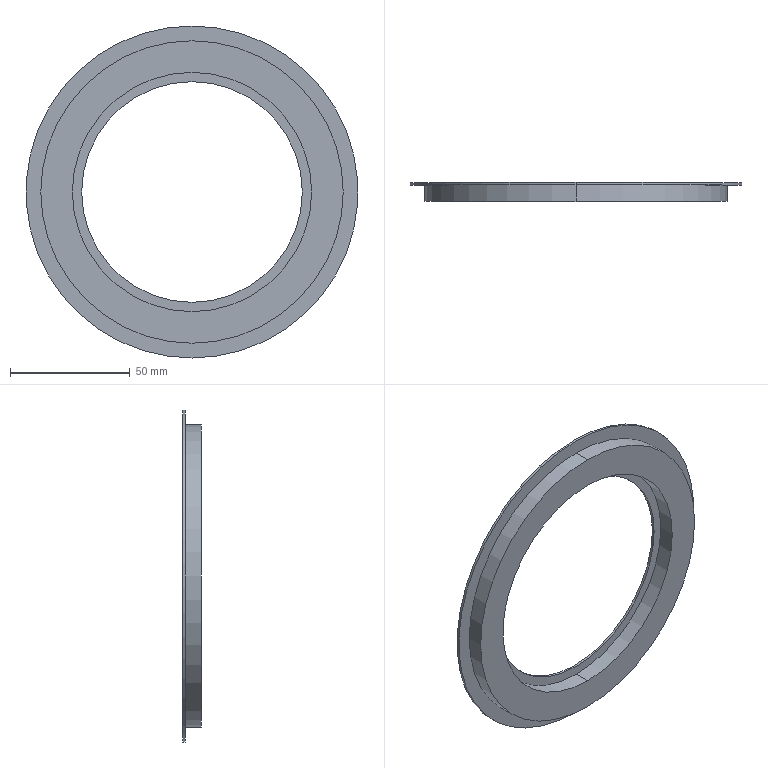Part | SolidWorks | features Revolution 1 | 2 solids | 18 faces | box 138.727 x 7.789 x 138.727 mm | volume 36485 mm3 | cylinder 12 | plane 6 | commonest cylinder face diameters 92.162 x2 100 x2 103.706 x2 124.067 x2 126.387 x2 138.727 x2
STEP:
#1=CARTESIAN_POINT('',(0.,160.532,69.363));
#2=VERTEX_POINT('',#1);
#3=CARTESIAN_POINT('',(0.,160.532,-69.363));
#4=VERTEX_POINT('',#3);
#5=CARTESIAN_POINT('',(0.,160.532,0.));
#6=DIRECTION('',(0.,1.,0.));
#7=DIRECTION('',(0.,0.,1.));
#8=AXIS2_PLACEMENT_3D('',#5,#6,#7);
#9=CIRCLE('',#8,69.363);
#10=EDGE_CURVE('',#2,#4,#9,.T.);
#11=ORIENTED_EDGE('',*,*,#10,.T.);
#12=CARTESIAN_POINT('',(0.,161.532,-69.363));
#13=VERTEX_POINT('',#12);
#14=CARTESIAN_POINT('',(0.,0.,-69.363));
#15=DIRECTION('',(0.,1.,0.));
#16=VECTOR('',#15,1000.);
#17=LINE('',#14,#16);
#18=EDGE_CURVE('',#4,#13,#17,.T.);
#19=ORIENTED_EDGE('',*,*,#18,.T.);
#20=CARTESIAN_POINT('',(0.,161.532,69.363));
#21=VERTEX_POINT('',#20);
#22=CARTESIAN_POINT('',(0.,161.532,0.));
#23=DIRECTION('',(0.,1.,0.));
#24=DIRECTION('',(0.,0.,1.));
#25=AXIS2_PLACEMENT_3D('',#22,#23,#24);
#26=CIRCLE('',#25,69.363);
#27=EDGE_CURVE('',#21,#13,#26,.T.);
#28=ORIENTED_EDGE('',*,*,#27,.F.);
#29=CARTESIAN_POINT('',(0.,0.,69.363));
#30=DIRECTION('',(0.,1.,0.));
#31=VECTOR('',#30,1000.);
#32=LINE('',#29,#31);
#33=EDGE_CURVE('',#2,#21,#32,.T.);
#34=ORIENTED_EDGE('',*,*,#33,.F.);
#35=EDGE_LOOP('',(#11,#19,#28,#34));
#36=FACE_OUTER_BOUND('',#35,.T.);
#37=CARTESIAN_POINT('',(0.,0.,0.));
#38=DIRECTION('',(0.,1.,0.));
#39=DIRECTION('',(0.,0.,1.));
#40=AXIS2_PLACEMENT_3D('',#37,#38,#39);
#41=CYLINDRICAL_SURFACE('',#40,69.363);
#42=ADVANCED_FACE('',(#36),#41,.T.);
#43=CARTESIAN_POINT('',(0.,160.532,-62.034));
#44=VERTEX_POINT('',#43);
#45=CARTESIAN_POINT('',(0.,160.532,62.034));
#46=VERTEX_POINT('',#45);
#47=CARTESIAN_POINT('',(0.,160.532,0.));
#48=DIRECTION('',(0.,1.,0.));
#49=DIRECTION('',(0.,0.,1.));
#50=AXIS2_PLACEMENT_3D('',#47,#48,#49);
#51=CIRCLE('',#50,62.034);
#52=EDGE_CURVE('',#44,#46,#51,.T.);
#53=ORIENTED_EDGE('',*,*,#52,.F.);
#54=CARTESIAN_POINT('',(0.,161.532,-62.034));
#55=VERTEX_POINT('',#54);
#56=CARTESIAN_POINT('',(0.,0.,-62.034));
#57=DIRECTION('',(0.,1.,0.));
#58=VECTOR('',#57,1000.);
#59=LINE('',#56,#58);
#60=EDGE_CURVE('',#44,#55,#59,.T.);
#61=ORIENTED_EDGE('',*,*,#60,.T.);
#62=CARTESIAN_POINT('',(0.,161.532,62.034));
#63=VERTEX_POINT('',#62);
#64=CARTESIAN_POINT('',(0.,161.532,0.));
#65=DIRECTION('',(0.,1.,0.));
#66=DIRECTION('',(0.,0.,1.));
#67=AXIS2_PLACEMENT_3D('',#64,#65,#66);
#68=CIRCLE('',#67,62.034);
#69=EDGE_CURVE('',#55,#63,#68,.T.);
#70=ORIENTED_EDGE('',*,*,#69,.T.);
#71=CARTESIAN_POINT('',(0.,0.,62.034));
#72=DIRECTION('',(0.,1.,0.));
#73=VECTOR('',#72,1000.);
#74=LINE('',#71,#73);
#75=EDGE_CURVE('',#46,#63,#74,.T.);
#76=ORIENTED_EDGE('',*,*,#75,.F.);
#77=EDGE_LOOP('',(#53,#61,#70,#76));
#78=FACE_OUTER_BOUND('',#77,.T.);
#79=CARTESIAN_POINT('',(0.,0.,0.));
#80=DIRECTION('',(0.,1.,0.));
#81=DIRECTION('',(0.,0.,1.));
#82=AXIS2_PLACEMENT_3D('',#79,#80,#81);
#83=CYLINDRICAL_SURFACE('',#82,62.034);
#84=ADVANCED_FACE('',(#78),#83,.F.);
#85=CARTESIAN_POINT('',(0.,153.779,-50.));
#86=VERTEX_POINT('',#85);
#87=CARTESIAN_POINT('',(0.,153.779,50.));
#88=VERTEX_POINT('',#87);
#89=CARTESIAN_POINT('',(0.,153.779,0.));
#90=DIRECTION('',(0.,1.,0.));
#91=DIRECTION('',(0.,0.,1.));
#92=AXIS2_PLACEMENT_3D('',#89,#90,#91);
#93=CIRCLE('',#92,50.);
#94=EDGE_CURVE('',#86,#88,#93,.T.);
#95=ORIENTED_EDGE('',*,*,#94,.F.);
#96=CARTESIAN_POINT('',(0.,160.532,-50.));
#97=VERTEX_POINT('',#96);
#98=CARTESIAN_POINT('',(0.,0.,-50.));
#99=DIRECTION('',(0.,1.,0.));
#100=VECTOR('',#99,1000.);
#101=LINE('',#98,#100);
#102=EDGE_CURVE('',#86,#97,#101,.T.);
#103=ORIENTED_EDGE('',*,*,#102,.T.);
#104=CARTESIAN_POINT('',(0.,160.532,50.));
#105=VERTEX_POINT('',#104);
#106=CARTESIAN_POINT('',(0.,160.532,0.));
#107=DIRECTION('',(0.,1.,0.));
#108=DIRECTION('',(0.,0.,1.));
#109=AXIS2_PLACEMENT_3D('',#106,#107,#108);
#110=CIRCLE('',#109,50.);
#111=EDGE_CURVE('',#97,#105,#110,.T.);
#112=ORIENTED_EDGE('',*,*,#111,.T.);
#113=CARTESIAN_POINT('',(0.,0.,50.));
#114=DIRECTION('',(0.,1.,0.));
#115=VECTOR('',#114,1000.);
#116=LINE('',#113,#115);
#117=EDGE_CURVE('',#88,#105,#116,.T.);
#118=ORIENTED_EDGE('',*,*,#117,.F.);
#119=EDGE_LOOP('',(#95,#103,#112,#118));
#120=FACE_OUTER_BOUND('',#119,.T.);
#121=CARTESIAN_POINT('',(0.,0.,0.));
#122=DIRECTION('',(0.,1.,0.));
#123=DIRECTION('',(0.,0.,1.));
#124=AXIS2_PLACEMENT_3D('',#121,#122,#123);
#125=CYLINDRICAL_SURFACE('',#124,50.);
#126=ADVANCED_FACE('',(#120),#125,.F.);
#127=CARTESIAN_POINT('',(0.,153.779,63.194));
#128=VERTEX_POINT('',#127);
#129=CARTESIAN_POINT('',(0.,153.779,-63.194));
#130=VERTEX_POINT('',#129);
#131=CARTESIAN_POINT('',(0.,153.779,0.));
#132=DIRECTION('',(0.,1.,0.));
#133=DIRECTION('',(0.,0.,1.));
#134=AXIS2_PLACEMENT_3D('',#131,#132,#133);
#135=CIRCLE('',#134,63.194);
#136=EDGE_CURVE('',#128,#130,#135,.T.);
#137=ORIENTED_EDGE('',*,*,#136,.T.);
#138=CARTESIAN_POINT('',(0.,160.532,-63.194));
#139=VERTEX_POINT('',#138);
#140=CARTESIAN_POINT('',(0.,0.,-63.194));
#141=DIRECTION('',(0.,1.,0.));
#142=VECTOR('',#141,1000.);
#143=LINE('',#140,#142);
#144=EDGE_CURVE('',#130,#139,#143,.T.);
#145=ORIENTED_EDGE('',*,*,#144,.T.);
#146=CARTESIAN_POINT('',(0.,160.532,63.194));
#147=VERTEX_POINT('',#146);
#148=CARTESIAN_POINT('',(0.,160.532,0.));
#149=DIRECTION('',(0.,1.,0.));
#150=DIRECTION('',(0.,0.,1.));
#151=AXIS2_PLACEMENT_3D('',#148,#149,#150);
#152=CIRCLE('',#151,63.194);
#153=EDGE_CURVE('',#147,#139,#152,.T.);
#154=ORIENTED_EDGE('',*,*,#153,.F.);
#155=CARTESIAN_POINT('',(0.,0.,63.194));
#156=DIRECTION('',(0.,1.,0.));
#157=VECTOR('',#156,1000.);
#158=LINE('',#155,#157);
#159=EDGE_CURVE('',#128,#147,#158,.T.);
#160=ORIENTED_EDGE('',*,*,#159,.F.);
#161=EDGE_LOOP('',(#137,#145,#154,#160));
#162=FACE_OUTER_BOUND('',#161,.T.);
#163=CARTESIAN_POINT('',(0.,0.,0.));
#164=DIRECTION('',(0.,1.,0.));
#165=DIRECTION('',(0.,0.,1.));
#166=AXIS2_PLACEMENT_3D('',#163,#164,#165);
#167=CYLINDRICAL_SURFACE('',#166,63.194);
#168=ADVANCED_FACE('',(#162),#167,.T.);
#169=ORIENTED_EDGE('',*,*,#144,.F.);
#170=CARTESIAN_POINT('',(0.,153.779,0.));
#171=DIRECTION('',(0.,1.,0.));
#172=DIRECTION('',(0.,0.,1.));
#173=AXIS2_PLACEMENT_3D('',#170,#171,#172);
#174=CIRCLE('',#173,63.194);
#175=EDGE_CURVE('',#130,#128,#174,.T.);
#176=ORIENTED_EDGE('',*,*,#175,.T.);
#177=ORIENTED_EDGE('',*,*,#159,.T.);
#178=CARTESIAN_POINT('',(0.,160.532,0.));
#179=DIRECTION('',(0.,1.,0.));
#180=DIRECTION('',(0.,0.,1.));
#181=AXIS2_PLACEMENT_3D('',#178,#179,#180);
#182=CIRCLE('',#181,63.194);
#183=EDGE_CURVE('',#139,#147,#182,.T.);
#184=ORIENTED_EDGE('',*,*,#183,.F.);
#185=EDGE_LOOP('',(#169,#176,#177,#184));
#186=FACE_OUTER_BOUND('',#185,.T.);
#187=CARTESIAN_POINT('',(0.,0.,0.));
#188=DIRECTION('',(0.,1.,0.));
#189=DIRECTION('',(0.,0.,1.));
#190=AXIS2_PLACEMENT_3D('',#187,#188,#189);
#191=CYLINDRICAL_SURFACE('',#190,63.194);
#192=ADVANCED_FACE('',(#186),#191,.T.);
#193=ORIENTED_EDGE('',*,*,#136,.F.);
#194=ORIENTED_EDGE('',*,*,#175,.F.);
#195=EDGE_LOOP('',(#193,#194));
#196=FACE_OUTER_BOUND('',#195,.T.);
#197=CARTESIAN_POINT('',(0.,153.779,0.));
#198=DIRECTION('',(0.,1.,0.));
#199=DIRECTION('',(0.,0.,1.));
#200=AXIS2_PLACEMENT_3D('',#197,#198,#199);
#201=CIRCLE('',#200,50.);
#202=EDGE_CURVE('',#88,#86,#201,.T.);
#203=ORIENTED_EDGE('',*,*,#202,.T.);
#204=ORIENTED_EDGE('',*,*,#94,.T.);
#205=EDGE_LOOP('',(#203,#204));
#206=FACE_BOUND('',#205,.T.);
#207=CARTESIAN_POINT('',(63.194,153.779,0.));
#208=DIRECTION('',(0.,1.,0.));
#209=DIRECTION('',(0.,0.,1.));
#210=AXIS2_PLACEMENT_3D('',#207,#208,#209);
#211=PLANE('',#210);
#212=ADVANCED_FACE('',(#196,#206),#211,.F.);
#213=ORIENTED_EDGE('',*,*,#102,.F.);
#214=ORIENTED_EDGE('',*,*,#202,.F.);
#215=ORIENTED_EDGE('',*,*,#117,.T.);
#216=CARTESIAN_POINT('',(0.,160.532,0.));
#217=DIRECTION('',(0.,1.,0.));
#218=DIRECTION('',(0.,0.,1.));
#219=AXIS2_PLACEMENT_3D('',#216,#217,#218);
#220=CIRCLE('',#219,50.);
#221=EDGE_CURVE('',#105,#97,#220,.T.);
#222=ORIENTED_EDGE('',*,*,#221,.T.);
#223=EDGE_LOOP('',(#213,#214,#215,#222));
#224=FACE_OUTER_BOUND('',#223,.T.);
#225=CARTESIAN_POINT('',(0.,0.,0.));
#226=DIRECTION('',(0.,1.,0.));
#227=DIRECTION('',(0.,0.,1.));
#228=AXIS2_PLACEMENT_3D('',#225,#226,#227);
#229=CYLINDRICAL_SURFACE('',#228,50.);
#230=ADVANCED_FACE('',(#224),#229,.F.);
#231=ORIENTED_EDGE('',*,*,#221,.F.);
#232=ORIENTED_EDGE('',*,*,#111,.F.);
#233=EDGE_LOOP('',(#231,#232));
#234=FACE_BOUND('',#233,.T.);
#235=CARTESIAN_POINT('',(0.,160.532,0.));
#236=DIRECTION('',(0.,1.,0.));
#237=DIRECTION('',(0.,0.,1.));
#238=AXIS2_PLACEMENT_3D('',#235,#236,#237);
#239=CIRCLE('',#238,62.034);
#240=EDGE_CURVE('',#46,#44,#239,.T.);
#241=ORIENTED_EDGE('',*,*,#240,.T.);
#242=ORIENTED_EDGE('',*,*,#52,.T.);
#243=EDGE_LOOP('',(#241,#242));
#244=FACE_OUTER_BOUND('',#243,.T.);
#245=CARTESIAN_POINT('',(50.,160.532,0.));
#246=DIRECTION('',(0.,-1.,0.));
#247=DIRECTION('',(0.,0.,-1.));
#248=AXIS2_PLACEMENT_3D('',#245,#246,#247);
#249=PLANE('',#248);
#250=ADVANCED_FACE('',(#234,#244),#249,.F.);
#251=ORIENTED_EDGE('',*,*,#60,.F.);
#252=ORIENTED_EDGE('',*,*,#240,.F.);
#253=ORIENTED_EDGE('',*,*,#75,.T.);
#254=CARTESIAN_POINT('',(0.,161.532,0.));
#255=DIRECTION('',(0.,1.,0.));
#256=DIRECTION('',(0.,0.,1.));
#257=AXIS2_PLACEMENT_3D('',#254,#255,#256);
#258=CIRCLE('',#257,62.034);
#259=EDGE_CURVE('',#63,#55,#258,.T.);
#260=ORIENTED_EDGE('',*,*,#259,.T.);
#261=EDGE_LOOP('',(#251,#252,#253,#260));
#262=FACE_OUTER_BOUND('',#261,.T.);
#263=CARTESIAN_POINT('',(0.,0.,0.));
#264=DIRECTION('',(0.,1.,0.));
#265=DIRECTION('',(0.,0.,1.));
#266=AXIS2_PLACEMENT_3D('',#263,#264,#265);
#267=CYLINDRICAL_SURFACE('',#266,62.034);
#268=ADVANCED_FACE('',(#262),#267,.F.);
#269=ORIENTED_EDGE('',*,*,#259,.F.);
#270=ORIENTED_EDGE('',*,*,#69,.F.);
#271=EDGE_LOOP('',(#269,#270));
#272=FACE_BOUND('',#271,.T.);
#273=ORIENTED_EDGE('',*,*,#27,.T.);
#274=CARTESIAN_POINT('',(0.,161.532,0.));
#275=DIRECTION('',(0.,1.,0.));
#276=DIRECTION('',(0.,0.,1.));
#277=AXIS2_PLACEMENT_3D('',#274,#275,#276);
#278=CIRCLE('',#277,69.363);
#279=EDGE_CURVE('',#13,#21,#278,.T.);
#280=ORIENTED_EDGE('',*,*,#279,.T.);
#281=EDGE_LOOP('',(#273,#280));
#282=FACE_OUTER_BOUND('',#281,.T.);
#283=CARTESIAN_POINT('',(69.363,161.532,0.));
#284=DIRECTION('',(0.,-1.,0.));
#285=DIRECTION('',(0.,0.,-1.));
#286=AXIS2_PLACEMENT_3D('',#283,#284,#285);
#287=PLANE('',#286);
#288=ADVANCED_FACE('',(#272,#282),#287,.F.);
#289=ORIENTED_EDGE('',*,*,#18,.F.);
#290=CARTESIAN_POINT('',(0.,160.532,0.));
#291=DIRECTION('',(0.,1.,0.));
#292=DIRECTION('',(0.,0.,1.));
#293=AXIS2_PLACEMENT_3D('',#290,#291,#292);
#294=CIRCLE('',#293,69.363);
#295=EDGE_CURVE('',#4,#2,#294,.T.);
#296=ORIENTED_EDGE('',*,*,#295,.T.);
#297=ORIENTED_EDGE('',*,*,#33,.T.);
#298=ORIENTED_EDGE('',*,*,#279,.F.);
#299=EDGE_LOOP('',(#289,#296,#297,#298));
#300=FACE_OUTER_BOUND('',#299,.T.);
#301=CARTESIAN_POINT('',(0.,0.,0.));
#302=DIRECTION('',(0.,1.,0.));
#303=DIRECTION('',(0.,0.,1.));
#304=AXIS2_PLACEMENT_3D('',#301,#302,#303);
#305=CYLINDRICAL_SURFACE('',#304,69.363);
#306=ADVANCED_FACE('',(#300),#305,.T.);
#307=ORIENTED_EDGE('',*,*,#10,.F.);
#308=ORIENTED_EDGE('',*,*,#295,.F.);
#309=EDGE_LOOP('',(#307,#308));
#310=FACE_OUTER_BOUND('',#309,.T.);
#311=ORIENTED_EDGE('',*,*,#153,.T.);
#312=ORIENTED_EDGE('',*,*,#183,.T.);
#313=EDGE_LOOP('',(#311,#312));
#314=FACE_BOUND('',#313,.T.);
#315=CARTESIAN_POINT('',(63.194,160.532,0.));
#316=DIRECTION('',(0.,1.,0.));
#317=DIRECTION('',(0.,0.,1.));
#318=AXIS2_PLACEMENT_3D('',#315,#316,#317);
#319=PLANE('',#318);
#320=ADVANCED_FACE('',(#310,#314),#319,.F.);
#321=CLOSED_SHELL('',(#42,#84,#126,#168,#192,#212,#230,#250,#268,#288,#306,#320));
#322=MANIFOLD_SOLID_BREP('',#321);
#323=CARTESIAN_POINT('',(0.,160.568,51.853));
#324=VERTEX_POINT('',#323);
#325=CARTESIAN_POINT('',(0.,160.568,-51.853));
#326=VERTEX_POINT('',#325);
#327=CARTESIAN_POINT('',(0.,160.568,0.));
#328=DIRECTION('',(0.,1.,0.));
#329=DIRECTION('',(0.,0.,1.));
#330=AXIS2_PLACEMENT_3D('',#327,#328,#329);
#331=CIRCLE('',#330,51.853);
#332=EDGE_CURVE('',#324,#326,#331,.T.);
#333=ORIENTED_EDGE('',*,*,#332,.T.);
#334=CARTESIAN_POINT('',(0.,161.568,-51.853));
#335=VERTEX_POINT('',#334);
#336=CARTESIAN_POINT('',(0.,0.,-51.853));
#337=DIRECTION('',(0.,1.,0.));
#338=VECTOR('',#337,1000.);
#339=LINE('',#336,#338);
#340=EDGE_CURVE('',#326,#335,#339,.T.);
#341=ORIENTED_EDGE('',*,*,#340,.T.);
#342=CARTESIAN_POINT('',(0.,161.568,51.853));
#343=VERTEX_POINT('',#342);
#344=CARTESIAN_POINT('',(0.,161.568,0.));
#345=DIRECTION('',(0.,1.,0.));
#346=DIRECTION('',(0.,0.,1.));
#347=AXIS2_PLACEMENT_3D('',#344,#345,#346);
#348=CIRCLE('',#347,51.853);
#349=EDGE_CURVE('',#343,#335,#348,.T.);
#350=ORIENTED_EDGE('',*,*,#349,.F.);
#351=CARTESIAN_POINT('',(0.,0.,51.853));
#352=DIRECTION('',(0.,1.,0.));
#353=VECTOR('',#352,1000.);
#354=LINE('',#351,#353);
#355=EDGE_CURVE('',#324,#343,#354,.T.);
#356=ORIENTED_EDGE('',*,*,#355,.F.);
#357=EDGE_LOOP('',(#333,#341,#350,#356));
#358=FACE_OUTER_BOUND('',#357,.T.);
#359=CARTESIAN_POINT('',(0.,0.,0.));
#360=DIRECTION('',(0.,1.,0.));
#361=DIRECTION('',(0.,0.,1.));
#362=AXIS2_PLACEMENT_3D('',#359,#360,#361);
#363=CYLINDRICAL_SURFACE('',#362,51.853);
#364=ADVANCED_FACE('',(#358),#363,.T.);
#365=CARTESIAN_POINT('',(0.,160.568,-46.081));
#366=VERTEX_POINT('',#365);
#367=CARTESIAN_POINT('',(0.,160.568,46.081));
#368=VERTEX_POINT('',#367);
#369=CARTESIAN_POINT('',(0.,160.568,0.));
#370=DIRECTION('',(0.,1.,0.));
#371=DIRECTION('',(0.,0.,1.));
#372=AXIS2_PLACEMENT_3D('',#369,#370,#371);
#373=CIRCLE('',#372,46.081);
#374=EDGE_CURVE('',#366,#368,#373,.T.);
#375=ORIENTED_EDGE('',*,*,#374,.F.);
#376=CARTESIAN_POINT('',(0.,161.568,-46.081));
#377=VERTEX_POINT('',#376);
#378=CARTESIAN_POINT('',(0.,0.,-46.081));
#379=DIRECTION('',(0.,1.,0.));
#380=VECTOR('',#379,1000.);
#381=LINE('',#378,#380);
#382=EDGE_CURVE('',#366,#377,#381,.T.);
#383=ORIENTED_EDGE('',*,*,#382,.T.);
#384=CARTESIAN_POINT('',(0.,161.568,46.081));
#385=VERTEX_POINT('',#384);
#386=CARTESIAN_POINT('',(0.,161.568,0.));
#387=DIRECTION('',(0.,1.,0.));
#388=DIRECTION('',(0.,0.,1.));
#389=AXIS2_PLACEMENT_3D('',#386,#387,#388);
#390=CIRCLE('',#389,46.081);
#391=EDGE_CURVE('',#377,#385,#390,.T.);
#392=ORIENTED_EDGE('',*,*,#391,.T.);
#393=CARTESIAN_POINT('',(0.,0.,46.081));
#394=DIRECTION('',(0.,1.,0.));
#395=VECTOR('',#394,1000.);
#396=LINE('',#393,#395);
#397=EDGE_CURVE('',#368,#385,#396,.T.);
#398=ORIENTED_EDGE('',*,*,#397,.F.);
#399=EDGE_LOOP('',(#375,#383,#392,#398));
#400=FACE_OUTER_BOUND('',#399,.T.);
#401=CARTESIAN_POINT('',(0.,0.,0.));
#402=DIRECTION('',(0.,1.,0.));
#403=DIRECTION('',(0.,0.,1.));
#404=AXIS2_PLACEMENT_3D('',#401,#402,#403);
#405=CYLINDRICAL_SURFACE('',#404,46.081);
#406=ADVANCED_FACE('',(#400),#405,.F.);
#407=ORIENTED_EDGE('',*,*,#382,.F.);
#408=CARTESIAN_POINT('',(0.,160.568,0.));
#409=DIRECTION('',(0.,1.,0.));
#410=DIRECTION('',(0.,0.,1.));
#411=AXIS2_PLACEMENT_3D('',#408,#409,#410);
#412=CIRCLE('',#411,46.081);
#413=EDGE_CURVE('',#368,#366,#412,.T.);
#414=ORIENTED_EDGE('',*,*,#413,.F.);
#415=ORIENTED_EDGE('',*,*,#397,.T.);
#416=CARTESIAN_POINT('',(0.,161.568,0.));
#417=DIRECTION('',(0.,1.,0.));
#418=DIRECTION('',(0.,0.,1.));
#419=AXIS2_PLACEMENT_3D('',#416,#417,#418);
#420=CIRCLE('',#419,46.081);
#421=EDGE_CURVE('',#385,#377,#420,.T.);
#422=ORIENTED_EDGE('',*,*,#421,.T.);
#423=EDGE_LOOP('',(#407,#414,#415,#422));
#424=FACE_OUTER_BOUND('',#423,.T.);
#425=CARTESIAN_POINT('',(0.,0.,0.));
#426=DIRECTION('',(0.,1.,0.));
#427=DIRECTION('',(0.,0.,1.));
#428=AXIS2_PLACEMENT_3D('',#425,#426,#427);
#429=CYLINDRICAL_SURFACE('',#428,46.081);
#430=ADVANCED_FACE('',(#424),#429,.F.);
#431=ORIENTED_EDGE('',*,*,#421,.F.);
#432=ORIENTED_EDGE('',*,*,#391,.F.);
#433=EDGE_LOOP('',(#431,#432));
#434=FACE_BOUND('',#433,.T.);
#435=ORIENTED_EDGE('',*,*,#349,.T.);
#436=CARTESIAN_POINT('',(0.,161.568,0.));
#437=DIRECTION('',(0.,1.,0.));
#438=DIRECTION('',(0.,0.,1.));
#439=AXIS2_PLACEMENT_3D('',#436,#437,#438);
#440=CIRCLE('',#439,51.853);
#441=EDGE_CURVE('',#335,#343,#440,.T.);
#442=ORIENTED_EDGE('',*,*,#441,.T.);
#443=EDGE_LOOP('',(#435,#442));
#444=FACE_OUTER_BOUND('',#443,.T.);
#445=CARTESIAN_POINT('',(46.081,161.568,0.));
#446=DIRECTION('',(0.,-1.,0.));
#447=DIRECTION('',(0.,0.,-1.));
#448=AXIS2_PLACEMENT_3D('',#445,#446,#447);
#449=PLANE('',#448);
#450=ADVANCED_FACE('',(#434,#444),#449,.F.);
#451=ORIENTED_EDGE('',*,*,#340,.F.);
#452=CARTESIAN_POINT('',(0.,160.568,0.));
#453=DIRECTION('',(0.,1.,0.));
#454=DIRECTION('',(0.,0.,1.));
#455=AXIS2_PLACEMENT_3D('',#452,#453,#454);
#456=CIRCLE('',#455,51.853);
#457=EDGE_CURVE('',#326,#324,#456,.T.);
#458=ORIENTED_EDGE('',*,*,#457,.T.);
#459=ORIENTED_EDGE('',*,*,#355,.T.);
#460=ORIENTED_EDGE('',*,*,#441,.F.);
#461=EDGE_LOOP('',(#451,#458,#459,#460));
#462=FACE_OUTER_BOUND('',#461,.T.);
#463=CARTESIAN_POINT('',(0.,0.,0.));
#464=DIRECTION('',(0.,1.,0.));
#465=DIRECTION('',(0.,0.,1.));
#466=AXIS2_PLACEMENT_3D('',#463,#464,#465);
#467=CYLINDRICAL_SURFACE('',#466,51.853);
#468=ADVANCED_FACE('',(#462),#467,.T.);
#469=ORIENTED_EDGE('',*,*,#332,.F.);
#470=ORIENTED_EDGE('',*,*,#457,.F.);
#471=EDGE_LOOP('',(#469,#470));
#472=FACE_OUTER_BOUND('',#471,.T.);
#473=ORIENTED_EDGE('',*,*,#413,.T.);
#474=ORIENTED_EDGE('',*,*,#374,.T.);
#475=EDGE_LOOP('',(#473,#474));
#476=FACE_BOUND('',#475,.T.);
#477=CARTESIAN_POINT('',(46.081,160.568,0.));
#478=DIRECTION('',(0.,1.,0.));
#479=DIRECTION('',(0.,0.,1.));
#480=AXIS2_PLACEMENT_3D('',#477,#478,#479);
#481=PLANE('',#480);
#482=ADVANCED_FACE('',(#472,#476),#481,.F.);
#483=CLOSED_SHELL('',(#364,#406,#430,#450,#468,#482));
#484=MANIFOLD_SOLID_BREP('',#483);
#485=CARTESIAN_POINT('',(0.,0.,0.));
#486=DIRECTION('',(0.,0.,1.));
#487=DIRECTION('',(1.,0.,0.));
#488=AXIS2_PLACEMENT_3D('',#485,#486,#487);
#489=(LENGTH_UNIT()NAMED_UNIT(*)SI_UNIT(.MILLI.,.METRE.));
#490=UNCERTAINTY_MEASURE_WITH_UNIT(LENGTH_MEASURE(0.00001),#489,'','');
#491=(NAMED_UNIT(*)PLANE_ANGLE_UNIT()SI_UNIT($,.RADIAN.));
#492=(NAMED_UNIT(*)SI_UNIT($,.STERADIAN.)SOLID_ANGLE_UNIT());
#493=(GEOMETRIC_REPRESENTATION_CONTEXT(3)GLOBAL_UNCERTAINTY_ASSIGNED_CONTEXT((#490))GLOBAL_UNIT_ASSIGNED_CONTEXT((#489,#491,#492))REPRESENTATION_CONTEXT('',''));
#494=ADVANCED_BREP_SHAPE_REPRESENTATION('',(#322,#484,#488),#493);